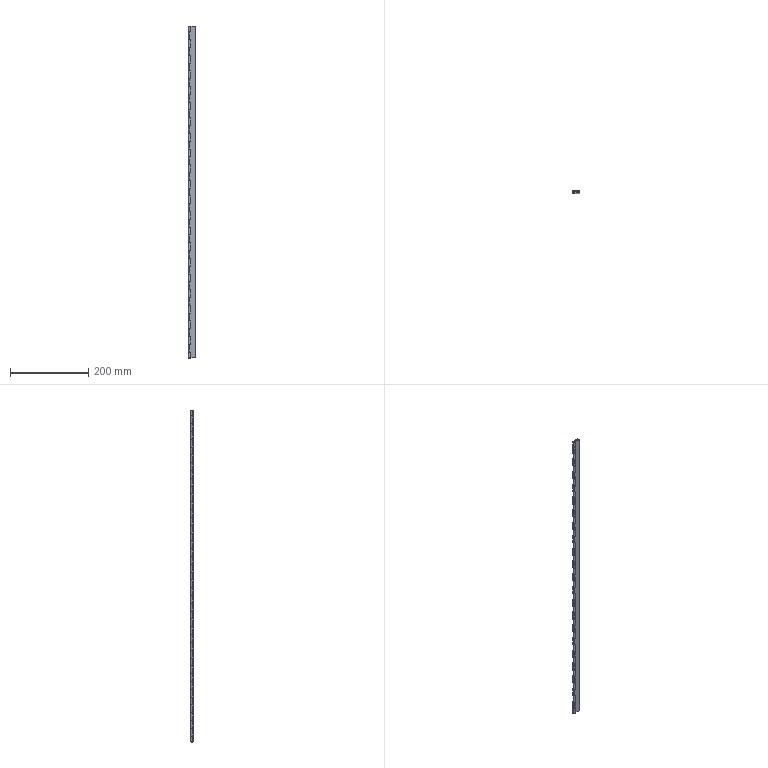Part | SolidWorks | features AEMSimFeature 1 | 3 solids | 360 faces | box 19.25 x 6.5 x 850 mm | volume 61984 mm3 | cylinder 217 | plane 139 | cone 4 | commonest cylinder face diameters 6.5 x129 3.5 x88